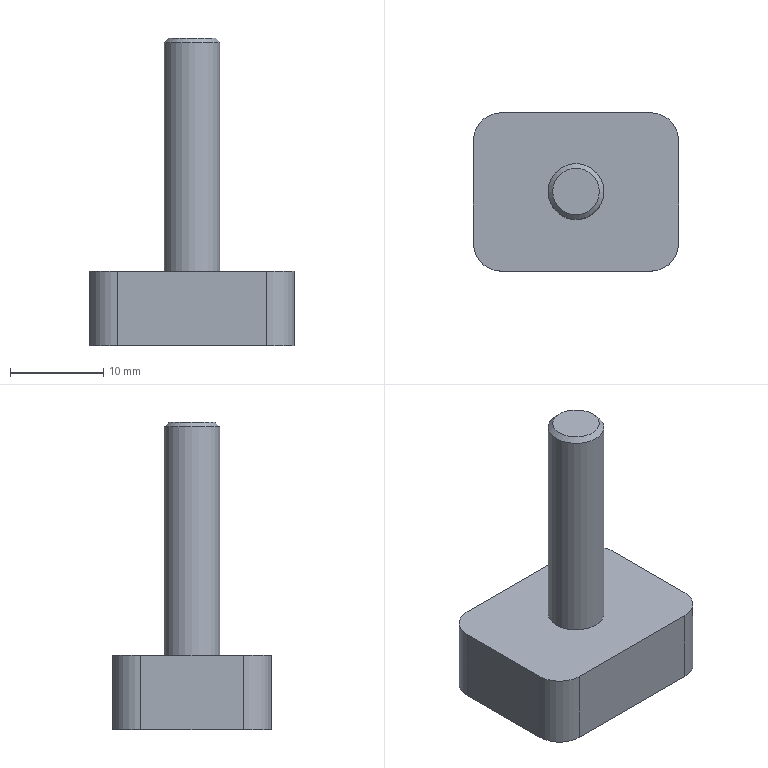Part | NX | features BREP 1 | 1 solid | 13 faces | box 22 x 17 x 33 mm | volume 3635 mm3 | plane 7 | cylinder 5 | cone 1 | commonest cylinder face diameters 6 x5
STEP:
#1=CARTESIAN_POINT('',(3.,0.,32.5));
#2=VERTEX_POINT('',#1);
#3=CARTESIAN_POINT('',(0.,0.,32.5));
#4=DIRECTION('',(0.,0.,-1.));
#5=DIRECTION('',(1.,0.,0.));
#6=AXIS2_PLACEMENT_3D('',#3,#4,#5);
#7=CIRCLE('',#6,3.);
#8=EDGE_CURVE('',#2,#2,#7,.T.);
#9=ORIENTED_EDGE('',*,*,#8,.F.);
#10=EDGE_LOOP('',(#9));
#11=FACE_BOUND('',#10,.T.);
#12=CARTESIAN_POINT('',(2.5,0.,33.));
#13=VERTEX_POINT('',#12);
#14=CARTESIAN_POINT('',(0.,0.,33.));
#15=DIRECTION('',(0.,0.,1.));
#16=DIRECTION('',(1.,0.,0.));
#17=AXIS2_PLACEMENT_3D('',#14,#15,#16);
#18=CIRCLE('',#17,2.5);
#19=EDGE_CURVE('',#13,#13,#18,.T.);
#20=ORIENTED_EDGE('',*,*,#19,.F.);
#21=EDGE_LOOP('',(#20));
#22=FACE_BOUND('',#21,.T.);
#23=CARTESIAN_POINT('',(0.,0.,33.));
#24=DIRECTION('',(0.,0.,-1.));
#25=DIRECTION('',(-1.,0.,0.));
#26=AXIS2_PLACEMENT_3D('',#23,#24,#25);
#27=CONICAL_SURFACE('',#26,2.5,0.7854);
#28=ADVANCED_FACE('',(#11,#22),#27,.T.);
#29=CARTESIAN_POINT('',(-3.,0.,8.));
#30=VERTEX_POINT('',#29);
#31=CARTESIAN_POINT('',(0.,0.,8.));
#32=DIRECTION('',(0.,0.,1.));
#33=DIRECTION('',(-1.,0.,0.));
#34=AXIS2_PLACEMENT_3D('',#31,#32,#33);
#35=CIRCLE('',#34,3.);
#36=EDGE_CURVE('',#30,#30,#35,.T.);
#37=ORIENTED_EDGE('',*,*,#36,.T.);
#38=EDGE_LOOP('',(#37));
#39=FACE_BOUND('',#38,.T.);
#40=ORIENTED_EDGE('',*,*,#8,.T.);
#41=EDGE_LOOP('',(#40));
#42=FACE_BOUND('',#41,.T.);
#43=CARTESIAN_POINT('',(0.,0.,33.));
#44=DIRECTION('',(0.,0.,-1.));
#45=DIRECTION('',(-1.,0.,0.));
#46=AXIS2_PLACEMENT_3D('',#43,#44,#45);
#47=CYLINDRICAL_SURFACE('',#46,3.);
#48=ADVANCED_FACE('',(#39,#42),#47,.T.);
#49=CARTESIAN_POINT('',(11.,-5.5,8.));
#50=VERTEX_POINT('',#49);
#51=CARTESIAN_POINT('',(11.,5.5,8.));
#52=VERTEX_POINT('',#51);
#53=CARTESIAN_POINT('',(11.,-8.5,8.));
#54=DIRECTION('',(0.,1.,0.));
#55=VECTOR('',#54,1000.);
#56=LINE('',#53,#55);
#57=EDGE_CURVE('',#50,#52,#56,.T.);
#58=ORIENTED_EDGE('',*,*,#57,.T.);
#59=CARTESIAN_POINT('',(8.,8.5,8.));
#60=VERTEX_POINT('',#59);
#61=CARTESIAN_POINT('',(8.,5.5,8.));
#62=DIRECTION('',(0.,0.,1.));
#63=DIRECTION('',(-1.,0.,0.));
#64=AXIS2_PLACEMENT_3D('',#61,#62,#63);
#65=CIRCLE('',#64,3.);
#66=EDGE_CURVE('',#52,#60,#65,.T.);
#67=ORIENTED_EDGE('',*,*,#66,.T.);
#68=CARTESIAN_POINT('',(-8.,8.5,8.));
#69=VERTEX_POINT('',#68);
#70=CARTESIAN_POINT('',(-11.,8.5,8.));
#71=DIRECTION('',(-1.,0.,0.));
#72=VECTOR('',#71,1000.);
#73=LINE('',#70,#72);
#74=EDGE_CURVE('',#60,#69,#73,.T.);
#75=ORIENTED_EDGE('',*,*,#74,.T.);
#76=CARTESIAN_POINT('',(-11.,5.5,8.));
#77=VERTEX_POINT('',#76);
#78=CARTESIAN_POINT('',(-8.,5.5,8.));
#79=DIRECTION('',(0.,0.,1.));
#80=DIRECTION('',(-1.,0.,0.));
#81=AXIS2_PLACEMENT_3D('',#78,#79,#80);
#82=CIRCLE('',#81,3.);
#83=EDGE_CURVE('',#69,#77,#82,.T.);
#84=ORIENTED_EDGE('',*,*,#83,.T.);
#85=CARTESIAN_POINT('',(-11.,-5.5,8.));
#86=VERTEX_POINT('',#85);
#87=CARTESIAN_POINT('',(-11.,-8.5,8.));
#88=DIRECTION('',(0.,-1.,0.));
#89=VECTOR('',#88,1000.);
#90=LINE('',#87,#89);
#91=EDGE_CURVE('',#77,#86,#90,.T.);
#92=ORIENTED_EDGE('',*,*,#91,.T.);
#93=CARTESIAN_POINT('',(-8.,-8.5,8.));
#94=VERTEX_POINT('',#93);
#95=CARTESIAN_POINT('',(-8.,-5.5,8.));
#96=DIRECTION('',(0.,0.,1.));
#97=DIRECTION('',(-1.,0.,0.));
#98=AXIS2_PLACEMENT_3D('',#95,#96,#97);
#99=CIRCLE('',#98,3.);
#100=EDGE_CURVE('',#86,#94,#99,.T.);
#101=ORIENTED_EDGE('',*,*,#100,.T.);
#102=CARTESIAN_POINT('',(8.,-8.5,8.));
#103=VERTEX_POINT('',#102);
#104=CARTESIAN_POINT('',(-11.,-8.5,8.));
#105=DIRECTION('',(1.,0.,0.));
#106=VECTOR('',#105,1000.);
#107=LINE('',#104,#106);
#108=EDGE_CURVE('',#94,#103,#107,.T.);
#109=ORIENTED_EDGE('',*,*,#108,.T.);
#110=CARTESIAN_POINT('',(8.,-5.5,8.));
#111=DIRECTION('',(0.,0.,1.));
#112=DIRECTION('',(-1.,0.,0.));
#113=AXIS2_PLACEMENT_3D('',#110,#111,#112);
#114=CIRCLE('',#113,3.);
#115=EDGE_CURVE('',#103,#50,#114,.T.);
#116=ORIENTED_EDGE('',*,*,#115,.T.);
#117=EDGE_LOOP('',(#58,#67,#75,#84,#92,#101,#109,#116));
#118=FACE_BOUND('',#117,.T.);
#119=ORIENTED_EDGE('',*,*,#36,.F.);
#120=EDGE_LOOP('',(#119));
#121=FACE_BOUND('',#120,.T.);
#122=CARTESIAN_POINT('',(0.,0.,8.));
#123=DIRECTION('',(0.,0.,-1.));
#124=DIRECTION('',(-1.,0.,0.));
#125=AXIS2_PLACEMENT_3D('',#122,#123,#124);
#126=PLANE('',#125);
#127=ADVANCED_FACE('',(#118,#121),#126,.F.);
#128=CARTESIAN_POINT('',(11.,-5.5,0.));
#129=VERTEX_POINT('',#128);
#130=CARTESIAN_POINT('',(11.,5.5,0.));
#131=VERTEX_POINT('',#130);
#132=CARTESIAN_POINT('',(11.,-8.5,0.));
#133=DIRECTION('',(0.,1.,0.));
#134=VECTOR('',#133,1000.);
#135=LINE('',#132,#134);
#136=EDGE_CURVE('',#129,#131,#135,.T.);
#137=ORIENTED_EDGE('',*,*,#136,.T.);
#138=CARTESIAN_POINT('',(11.,5.5,8.));
#139=DIRECTION('',(0.,0.,1.));
#140=VECTOR('',#139,1000.);
#141=LINE('',#138,#140);
#142=EDGE_CURVE('',#131,#52,#141,.T.);
#143=ORIENTED_EDGE('',*,*,#142,.T.);
#144=ORIENTED_EDGE('',*,*,#57,.F.);
#145=CARTESIAN_POINT('',(11.,-5.5,8.));
#146=DIRECTION('',(0.,0.,-1.));
#147=VECTOR('',#146,1000.);
#148=LINE('',#145,#147);
#149=EDGE_CURVE('',#50,#129,#148,.T.);
#150=ORIENTED_EDGE('',*,*,#149,.T.);
#151=EDGE_LOOP('',(#137,#143,#144,#150));
#152=FACE_BOUND('',#151,.T.);
#153=CARTESIAN_POINT('',(11.,-8.5,8.));
#154=DIRECTION('',(-1.,0.,0.));
#155=DIRECTION('',(0.,0.,1.));
#156=AXIS2_PLACEMENT_3D('',#153,#154,#155);
#157=PLANE('',#156);
#158=ADVANCED_FACE('',(#152),#157,.F.);
#159=ORIENTED_EDGE('',*,*,#74,.F.);
#160=CARTESIAN_POINT('',(8.,8.5,0.));
#161=VERTEX_POINT('',#160);
#162=CARTESIAN_POINT('',(8.,8.5,8.));
#163=DIRECTION('',(0.,0.,-1.));
#164=VECTOR('',#163,1000.);
#165=LINE('',#162,#164);
#166=EDGE_CURVE('',#60,#161,#165,.T.);
#167=ORIENTED_EDGE('',*,*,#166,.T.);
#168=CARTESIAN_POINT('',(-8.,8.5,0.));
#169=VERTEX_POINT('',#168);
#170=CARTESIAN_POINT('',(-11.,8.5,0.));
#171=DIRECTION('',(-1.,0.,0.));
#172=VECTOR('',#171,1000.);
#173=LINE('',#170,#172);
#174=EDGE_CURVE('',#161,#169,#173,.T.);
#175=ORIENTED_EDGE('',*,*,#174,.T.);
#176=CARTESIAN_POINT('',(-8.,8.5,8.));
#177=DIRECTION('',(0.,0.,1.));
#178=VECTOR('',#177,1000.);
#179=LINE('',#176,#178);
#180=EDGE_CURVE('',#169,#69,#179,.T.);
#181=ORIENTED_EDGE('',*,*,#180,.T.);
#182=EDGE_LOOP('',(#159,#167,#175,#181));
#183=FACE_BOUND('',#182,.T.);
#184=CARTESIAN_POINT('',(-11.,8.5,8.));
#185=DIRECTION('',(0.,-1.,0.));
#186=DIRECTION('',(0.,0.,-1.));
#187=AXIS2_PLACEMENT_3D('',#184,#185,#186);
#188=PLANE('',#187);
#189=ADVANCED_FACE('',(#183),#188,.F.);
#190=CARTESIAN_POINT('',(-11.,5.5,0.));
#191=VERTEX_POINT('',#190);
#192=CARTESIAN_POINT('',(-11.,-5.5,0.));
#193=VERTEX_POINT('',#192);
#194=CARTESIAN_POINT('',(-11.,-8.5,0.));
#195=DIRECTION('',(0.,-1.,0.));
#196=VECTOR('',#195,1000.);
#197=LINE('',#194,#196);
#198=EDGE_CURVE('',#191,#193,#197,.T.);
#199=ORIENTED_EDGE('',*,*,#198,.T.);
#200=CARTESIAN_POINT('',(-11.,-5.5,8.));
#201=DIRECTION('',(0.,0.,1.));
#202=VECTOR('',#201,1000.);
#203=LINE('',#200,#202);
#204=EDGE_CURVE('',#193,#86,#203,.T.);
#205=ORIENTED_EDGE('',*,*,#204,.T.);
#206=ORIENTED_EDGE('',*,*,#91,.F.);
#207=CARTESIAN_POINT('',(-11.,5.5,8.));
#208=DIRECTION('',(0.,0.,-1.));
#209=VECTOR('',#208,1000.);
#210=LINE('',#207,#209);
#211=EDGE_CURVE('',#77,#191,#210,.T.);
#212=ORIENTED_EDGE('',*,*,#211,.T.);
#213=EDGE_LOOP('',(#199,#205,#206,#212));
#214=FACE_BOUND('',#213,.T.);
#215=CARTESIAN_POINT('',(-11.,-8.5,8.));
#216=DIRECTION('',(1.,0.,0.));
#217=DIRECTION('',(0.,0.,-1.));
#218=AXIS2_PLACEMENT_3D('',#215,#216,#217);
#219=PLANE('',#218);
#220=ADVANCED_FACE('',(#214),#219,.F.);
#221=CARTESIAN_POINT('',(-8.,-8.5,0.));
#222=VERTEX_POINT('',#221);
#223=CARTESIAN_POINT('',(8.,-8.5,0.));
#224=VERTEX_POINT('',#223);
#225=CARTESIAN_POINT('',(-11.,-8.5,0.));
#226=DIRECTION('',(1.,0.,0.));
#227=VECTOR('',#226,1000.);
#228=LINE('',#225,#227);
#229=EDGE_CURVE('',#222,#224,#228,.T.);
#230=ORIENTED_EDGE('',*,*,#229,.T.);
#231=CARTESIAN_POINT('',(8.,-8.5,8.));
#232=DIRECTION('',(0.,0.,1.));
#233=VECTOR('',#232,1000.);
#234=LINE('',#231,#233);
#235=EDGE_CURVE('',#224,#103,#234,.T.);
#236=ORIENTED_EDGE('',*,*,#235,.T.);
#237=ORIENTED_EDGE('',*,*,#108,.F.);
#238=CARTESIAN_POINT('',(-8.,-8.5,8.));
#239=DIRECTION('',(0.,0.,-1.));
#240=VECTOR('',#239,1000.);
#241=LINE('',#238,#240);
#242=EDGE_CURVE('',#94,#222,#241,.T.);
#243=ORIENTED_EDGE('',*,*,#242,.T.);
#244=EDGE_LOOP('',(#230,#236,#237,#243));
#245=FACE_BOUND('',#244,.T.);
#246=CARTESIAN_POINT('',(-11.,-8.5,8.));
#247=DIRECTION('',(0.,1.,0.));
#248=DIRECTION('',(0.,0.,1.));
#249=AXIS2_PLACEMENT_3D('',#246,#247,#248);
#250=PLANE('',#249);
#251=ADVANCED_FACE('',(#245),#250,.F.);
#252=ORIENTED_EDGE('',*,*,#174,.F.);
#253=CARTESIAN_POINT('',(8.,5.5,0.));
#254=DIRECTION('',(0.,0.,-1.));
#255=DIRECTION('',(-1.,0.,0.));
#256=AXIS2_PLACEMENT_3D('',#253,#254,#255);
#257=CIRCLE('',#256,3.);
#258=EDGE_CURVE('',#161,#131,#257,.T.);
#259=ORIENTED_EDGE('',*,*,#258,.T.);
#260=ORIENTED_EDGE('',*,*,#136,.F.);
#261=CARTESIAN_POINT('',(8.,-5.5,0.));
#262=DIRECTION('',(0.,0.,-1.));
#263=DIRECTION('',(-1.,0.,0.));
#264=AXIS2_PLACEMENT_3D('',#261,#262,#263);
#265=CIRCLE('',#264,3.);
#266=EDGE_CURVE('',#129,#224,#265,.T.);
#267=ORIENTED_EDGE('',*,*,#266,.T.);
#268=ORIENTED_EDGE('',*,*,#229,.F.);
#269=CARTESIAN_POINT('',(-8.,-5.5,0.));
#270=DIRECTION('',(0.,0.,-1.));
#271=DIRECTION('',(-1.,0.,0.));
#272=AXIS2_PLACEMENT_3D('',#269,#270,#271);
#273=CIRCLE('',#272,3.);
#274=EDGE_CURVE('',#222,#193,#273,.T.);
#275=ORIENTED_EDGE('',*,*,#274,.T.);
#276=ORIENTED_EDGE('',*,*,#198,.F.);
#277=CARTESIAN_POINT('',(-8.,5.5,0.));
#278=DIRECTION('',(0.,0.,-1.));
#279=DIRECTION('',(-1.,0.,0.));
#280=AXIS2_PLACEMENT_3D('',#277,#278,#279);
#281=CIRCLE('',#280,3.);
#282=EDGE_CURVE('',#191,#169,#281,.T.);
#283=ORIENTED_EDGE('',*,*,#282,.T.);
#284=EDGE_LOOP('',(#252,#259,#260,#267,#268,#275,#276,#283));
#285=FACE_BOUND('',#284,.T.);
#286=CARTESIAN_POINT('',(0.,0.,0.));
#287=DIRECTION('',(0.,0.,-1.));
#288=DIRECTION('',(-1.,0.,0.));
#289=AXIS2_PLACEMENT_3D('',#286,#287,#288);
#290=PLANE('',#289);
#291=ADVANCED_FACE('',(#285),#290,.T.);
#292=ORIENTED_EDGE('',*,*,#66,.F.);
#293=ORIENTED_EDGE('',*,*,#142,.F.);
#294=ORIENTED_EDGE('',*,*,#258,.F.);
#295=ORIENTED_EDGE('',*,*,#166,.F.);
#296=EDGE_LOOP('',(#292,#293,#294,#295));
#297=FACE_BOUND('',#296,.T.);
#298=CARTESIAN_POINT('',(8.,5.5,8.));
#299=DIRECTION('',(0.,0.,-1.));
#300=DIRECTION('',(-1.,0.,0.));
#301=AXIS2_PLACEMENT_3D('',#298,#299,#300);
#302=CYLINDRICAL_SURFACE('',#301,3.);
#303=ADVANCED_FACE('',(#297),#302,.T.);
#304=ORIENTED_EDGE('',*,*,#115,.F.);
#305=ORIENTED_EDGE('',*,*,#235,.F.);
#306=ORIENTED_EDGE('',*,*,#266,.F.);
#307=ORIENTED_EDGE('',*,*,#149,.F.);
#308=EDGE_LOOP('',(#304,#305,#306,#307));
#309=FACE_BOUND('',#308,.T.);
#310=CARTESIAN_POINT('',(8.,-5.5,8.));
#311=DIRECTION('',(0.,0.,-1.));
#312=DIRECTION('',(-1.,0.,0.));
#313=AXIS2_PLACEMENT_3D('',#310,#311,#312);
#314=CYLINDRICAL_SURFACE('',#313,3.);
#315=ADVANCED_FACE('',(#309),#314,.T.);
#316=ORIENTED_EDGE('',*,*,#100,.F.);
#317=ORIENTED_EDGE('',*,*,#204,.F.);
#318=ORIENTED_EDGE('',*,*,#274,.F.);
#319=ORIENTED_EDGE('',*,*,#242,.F.);
#320=EDGE_LOOP('',(#316,#317,#318,#319));
#321=FACE_BOUND('',#320,.T.);
#322=CARTESIAN_POINT('',(-8.,-5.5,8.));
#323=DIRECTION('',(0.,0.,-1.));
#324=DIRECTION('',(-1.,0.,0.));
#325=AXIS2_PLACEMENT_3D('',#322,#323,#324);
#326=CYLINDRICAL_SURFACE('',#325,3.);
#327=ADVANCED_FACE('',(#321),#326,.T.);
#328=ORIENTED_EDGE('',*,*,#83,.F.);
#329=ORIENTED_EDGE('',*,*,#180,.F.);
#330=ORIENTED_EDGE('',*,*,#282,.F.);
#331=ORIENTED_EDGE('',*,*,#211,.F.);
#332=EDGE_LOOP('',(#328,#329,#330,#331));
#333=FACE_BOUND('',#332,.T.);
#334=CARTESIAN_POINT('',(-8.,5.5,8.));
#335=DIRECTION('',(0.,0.,-1.));
#336=DIRECTION('',(-1.,0.,0.));
#337=AXIS2_PLACEMENT_3D('',#334,#335,#336);
#338=CYLINDRICAL_SURFACE('',#337,3.);
#339=ADVANCED_FACE('',(#333),#338,.T.);
#340=ORIENTED_EDGE('',*,*,#19,.T.);
#341=EDGE_LOOP('',(#340));
#342=FACE_BOUND('',#341,.T.);
#343=CARTESIAN_POINT('',(0.,0.,33.));
#344=DIRECTION('',(0.,0.,1.));
#345=DIRECTION('',(1.,0.,0.));
#346=AXIS2_PLACEMENT_3D('',#343,#344,#345);
#347=PLANE('',#346);
#348=ADVANCED_FACE('',(#342),#347,.T.);
#349=CLOSED_SHELL('',(#28,#48,#127,#158,#189,#220,#251,#291,#303,#315,#327,#339,#348));
#350=MANIFOLD_SOLID_BREP('',#349);
#351=(LENGTH_UNIT()NAMED_UNIT(*)SI_UNIT(.MILLI.,.METRE.));
#352=UNCERTAINTY_MEASURE_WITH_UNIT(LENGTH_MEASURE(0.00001),#351,'','');
#353=(NAMED_UNIT(*)PLANE_ANGLE_UNIT()SI_UNIT($,.RADIAN.));
#354=(NAMED_UNIT(*)SI_UNIT($,.STERADIAN.)SOLID_ANGLE_UNIT());
#355=(GEOMETRIC_REPRESENTATION_CONTEXT(3)GLOBAL_UNCERTAINTY_ASSIGNED_CONTEXT((#352))GLOBAL_UNIT_ASSIGNED_CONTEXT((#351,#353,#354))REPRESENTATION_CONTEXT('',''));
#356=ADVANCED_BREP_SHAPE_REPRESENTATION('',(#350),#355);